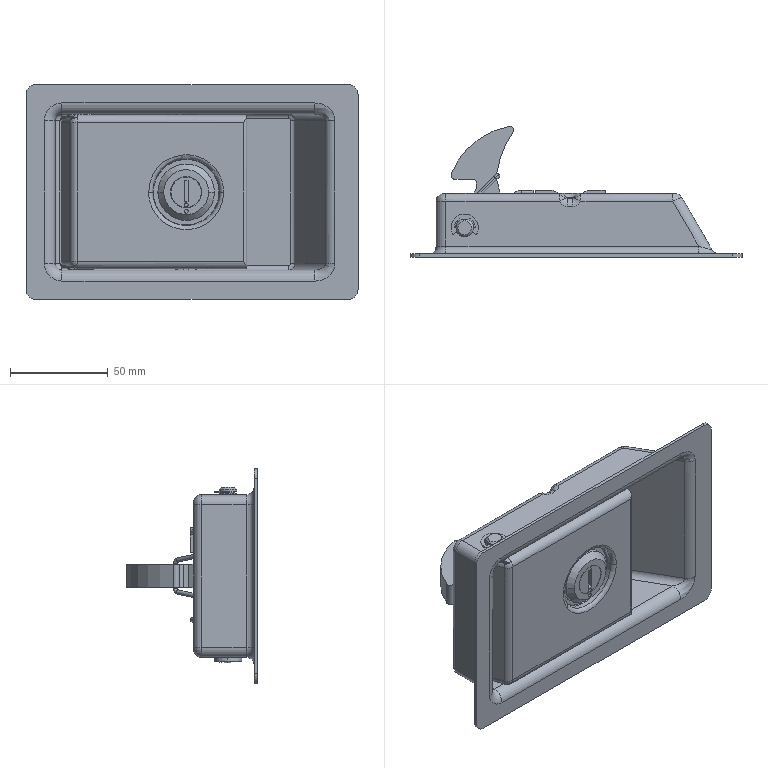Part | SolidWorks | features BaseBody 17 | 17 solids | 598 faces | box 170 x 67.2 x 110 mm | volume 99328 mm3 | plane 237 | cylinder 234 | torus 79 | sphere 23 | spline 16 | cone 9 | commonest cylinder face diameters 4 x26 8 x26 2 x17 4.8 x15 2.2 x14 10 x11